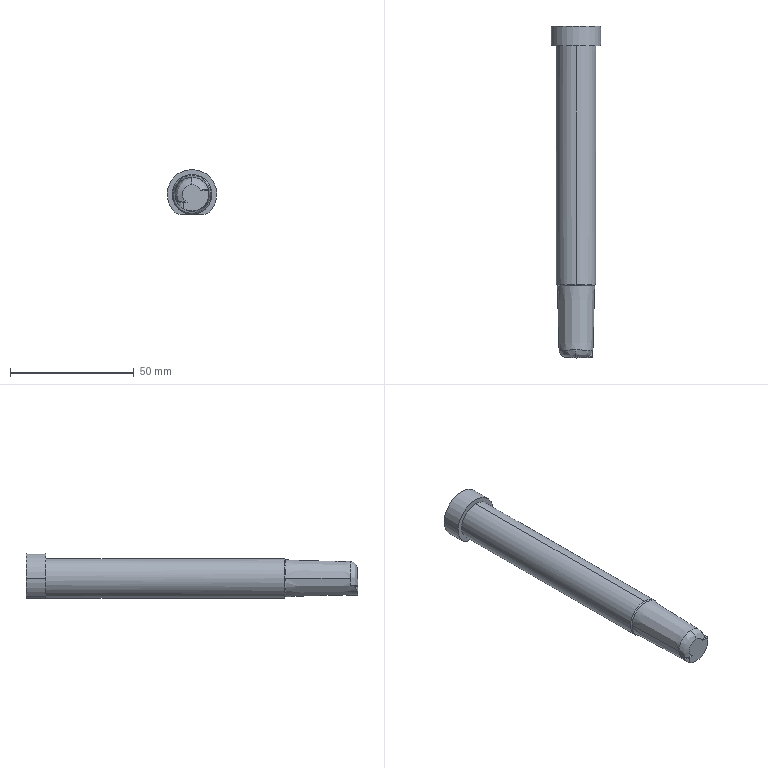Part | SolidWorks | features BaseBody 1 | 1 solid | 25 faces | box 20 x 134.117 x 18.065 mm | volume 26492 mm3 | cylinder 10 | plane 6 | spline 5 | cone 4 | commonest cylinder face diameters 20 x3 0.603 x2 6 x2 16 x2 6.033 x1
STEP:
#1=CARTESIAN_POINT('',(7.528,100.091,21.065));
#2=VERTEX_POINT('',#1);
#3=CARTESIAN_POINT('',(-7.528,100.091,21.065));
#4=VERTEX_POINT('',#3);
#5=CARTESIAN_POINT('',(0.,100.091,21.065));
#6=DIRECTION('',(0.,1.,0.));
#7=DIRECTION('',(1.,0.,0.));
#8=AXIS2_PLACEMENT_3D('',#5,#6,#7);
#9=CIRCLE('',#8,7.528);
#10=EDGE_CURVE('',#2,#4,#9,.T.);
#11=ORIENTED_EDGE('',*,*,#10,.T.);
#12=CARTESIAN_POINT('',(-8.,100.551,21.065));
#13=VERTEX_POINT('',#12);
#14=CARTESIAN_POINT('',(-8.044,100.594,21.065));
#15=DIRECTION('',(-0.7163,0.6978,0.));
#16=VECTOR('',#15,1000.);
#17=LINE('',#14,#16);
#18=EDGE_CURVE('',#4,#13,#17,.T.);
#19=ORIENTED_EDGE('',*,*,#18,.T.);
#20=CARTESIAN_POINT('',(0.,100.551,13.065));
#21=VERTEX_POINT('',#20);
#22=CARTESIAN_POINT('',(0.,100.551,21.065));
#23=DIRECTION('',(0.,1.,0.));
#24=DIRECTION('',(-1.,0.,0.));
#25=AXIS2_PLACEMENT_3D('',#22,#23,#24);
#26=CIRCLE('',#25,8.);
#27=EDGE_CURVE('',#21,#13,#26,.T.);
#28=ORIENTED_EDGE('',*,*,#27,.F.);
#29=CARTESIAN_POINT('',(8.,100.551,21.065));
#30=VERTEX_POINT('',#29);
#31=CARTESIAN_POINT('',(0.,100.551,21.065));
#32=DIRECTION('',(0.,1.,0.));
#33=DIRECTION('',(-1.,0.,0.));
#34=AXIS2_PLACEMENT_3D('',#31,#32,#33);
#35=CIRCLE('',#34,8.);
#36=EDGE_CURVE('',#30,#21,#35,.T.);
#37=ORIENTED_EDGE('',*,*,#36,.F.);
#38=CARTESIAN_POINT('',(8.044,100.594,21.065));
#39=DIRECTION('',(0.7163,0.6978,0.));
#40=VECTOR('',#39,1000.);
#41=LINE('',#38,#40);
#42=EDGE_CURVE('',#2,#30,#41,.T.);
#43=ORIENTED_EDGE('',*,*,#42,.F.);
#44=EDGE_LOOP('',(#11,#19,#28,#37,#43));
#45=FACE_OUTER_BOUND('',#44,.T.);
#46=CARTESIAN_POINT('',(0.,100.594,21.065));
#47=DIRECTION('',(0.,1.,0.));
#48=DIRECTION('',(1.,0.,0.));
#49=AXIS2_PLACEMENT_3D('',#46,#47,#48);
#50=CONICAL_SURFACE('',#49,8.044,0.7985);
#51=ADVANCED_FACE('',(#45),#50,.T.);
#52=CARTESIAN_POINT('',(-6.845,73.998,21.065));
#53=VERTEX_POINT('',#52);
#54=CARTESIAN_POINT('',(-6.191,73.956,18.149));
#55=VERTEX_POINT('',#54);
#56=CARTESIAN_POINT('',(-6.845,73.998,21.065));
#57=CARTESIAN_POINT('',(-6.845,73.991,20.559));
#58=CARTESIAN_POINT('',(-6.789,73.984,20.063));
#59=CARTESIAN_POINT('',(-6.571,73.969,19.088));
#60=CARTESIAN_POINT('',(-6.407,73.962,18.607));
#61=CARTESIAN_POINT('',(-6.191,73.956,18.149));
#62=B_SPLINE_CURVE_WITH_KNOTS('',3,(#56,#57,#58,#59,#60,#61),.UNSPECIFIED.,.F.,.F.,(4,2,4),(0.,0.001496,0.002993),.UNSPECIFIED.);
#63=EDGE_CURVE('',#53,#55,#62,.T.);
#64=ORIENTED_EDGE('',*,*,#63,.F.);
#65=CARTESIAN_POINT('',(-7.541,100.594,21.065));
#66=DIRECTION('',(-0.02618,0.9997,0.));
#67=VECTOR('',#66,1000.);
#68=LINE('',#65,#67);
#69=EDGE_CURVE('',#53,#4,#68,.T.);
#70=ORIENTED_EDGE('',*,*,#69,.T.);
#71=ORIENTED_EDGE('',*,*,#10,.F.);
#72=CARTESIAN_POINT('',(6.768,71.06,21.065));
#73=VERTEX_POINT('',#72);
#74=CARTESIAN_POINT('',(7.541,100.594,21.065));
#75=DIRECTION('',(0.02618,0.9997,0.));
#76=VECTOR('',#75,1000.);
#77=LINE('',#74,#76);
#78=EDGE_CURVE('',#73,#2,#77,.T.);
#79=ORIENTED_EDGE('',*,*,#78,.F.);
#80=CARTESIAN_POINT('',(-3.608,70.91,15.344));
#81=VERTEX_POINT('',#80);
#82=CARTESIAN_POINT('',(6.768,71.06,21.065));
#83=CARTESIAN_POINT('',(6.764,70.902,15.041));
#84=CARTESIAN_POINT('',(1.488,70.826,12.132));
#85=CARTESIAN_POINT('',(-3.608,70.91,15.344));
#86=(BOUNDED_CURVE()B_SPLINE_CURVE(3,(#82,#83,#84,#85),.UNSPECIFIED.,.F.,.F.)B_SPLINE_CURVE_WITH_KNOTS((4,4),(1.571,3.704),.UNSPECIFIED.)CURVE()GEOMETRIC_REPRESENTATION_ITEM()RATIONAL_B_SPLINE_CURVE((1.,0.6556,0.6556,1.))REPRESENTATION_ITEM(''));
#87=EDGE_CURVE('',#73,#81,#86,.T.);
#88=ORIENTED_EDGE('',*,*,#87,.T.);
#89=CARTESIAN_POINT('',(-5.995,72.237,17.859));
#90=VERTEX_POINT('',#89);
#91=CARTESIAN_POINT('',(-3.608,70.91,15.344));
#92=CARTESIAN_POINT('',(-3.879,70.914,15.515));
#93=CARTESIAN_POINT('',(-4.131,70.956,15.699));
#94=CARTESIAN_POINT('',(-4.603,71.094,16.093));
#95=CARTESIAN_POINT('',(-4.825,71.193,16.306));
#96=CARTESIAN_POINT('',(-5.224,71.428,16.737));
#97=CARTESIAN_POINT('',(-5.403,71.565,16.958));
#98=CARTESIAN_POINT('',(-5.725,71.875,17.406));
#99=CARTESIAN_POINT('',(-5.869,72.047,17.635));
#100=CARTESIAN_POINT('',(-5.995,72.237,17.859));
#101=B_SPLINE_CURVE_WITH_KNOTS('',3,(#91,#92,#93,#94,#95,#96,#97,#98,#99,#100),.UNSPECIFIED.,.F.,.F.,(4,2,2,2,4),(0.00007647,0.001021,0.001965,0.002909,0.003853),.UNSPECIFIED.);
#102=EDGE_CURVE('',#81,#90,#101,.T.);
#103=ORIENTED_EDGE('',*,*,#102,.T.);
#104=CARTESIAN_POINT('',(-6.169,73.191,18.148));
#105=VERTEX_POINT('',#104);
#106=CARTESIAN_POINT('',(-5.995,72.237,17.859));
#107=CARTESIAN_POINT('',(-6.03,72.289,17.921));
#108=CARTESIAN_POINT('',(-6.055,72.361,17.967));
#109=CARTESIAN_POINT('',(-6.097,72.513,18.04));
#110=CARTESIAN_POINT('',(-6.113,72.595,18.067));
#111=CARTESIAN_POINT('',(-6.15,72.846,18.128));
#112=CARTESIAN_POINT('',(-6.161,73.018,18.143));
#113=CARTESIAN_POINT('',(-6.169,73.191,18.148));
#114=B_SPLINE_CURVE_WITH_KNOTS('',3,(#106,#107,#108,#109,#110,#111,#112,#113),.UNSPECIFIED.,.F.,.F.,(4,2,2,4),(0.,0.0002617,0.0005235,0.001047),.UNSPECIFIED.);
#115=EDGE_CURVE('',#90,#105,#114,.T.);
#116=ORIENTED_EDGE('',*,*,#115,.T.);
#117=CARTESIAN_POINT('',(-6.173,73.305,18.149));
#118=VERTEX_POINT('',#117);
#119=CARTESIAN_POINT('',(-6.169,73.191,18.148));
#120=CARTESIAN_POINT('',(-6.17,73.229,18.149));
#121=CARTESIAN_POINT('',(-6.171,73.267,18.149));
#122=CARTESIAN_POINT('',(-6.173,73.305,18.149));
#123=B_SPLINE_CURVE_WITH_KNOTS('',3,(#119,#120,#121,#122),.UNSPECIFIED.,.F.,.F.,(4,4),(0.,0.000114),.UNSPECIFIED.);
#124=EDGE_CURVE('',#105,#118,#123,.T.);
#125=ORIENTED_EDGE('',*,*,#124,.T.);
#126=CARTESIAN_POINT('',(-6.173,73.305,18.149));
#127=CARTESIAN_POINT('',(-6.179,73.522,18.149));
#128=CARTESIAN_POINT('',(-6.185,73.739,18.149));
#129=CARTESIAN_POINT('',(-6.191,73.956,18.149));
#130=B_SPLINE_CURVE_WITH_KNOTS('',3,(#126,#127,#128,#129),.UNSPECIFIED.,.F.,.F.,(4,4),(0.03892,0.03957),.UNSPECIFIED.);
#131=EDGE_CURVE('',#118,#55,#130,.T.);
#132=ORIENTED_EDGE('',*,*,#131,.T.);
#133=EDGE_LOOP('',(#64,#70,#71,#79,#88,#103,#116,#125,#132));
#134=FACE_OUTER_BOUND('',#133,.T.);
#135=CARTESIAN_POINT('',(0.,100.594,21.065));
#136=DIRECTION('',(0.,1.,0.));
#137=DIRECTION('',(1.,0.,0.));
#138=AXIS2_PLACEMENT_3D('',#135,#136,#137);
#139=CONICAL_SURFACE('',#138,7.541,0.02618);
#140=ADVANCED_FACE('',(#134),#139,.T.);
#141=CARTESIAN_POINT('',(6.602,74.025,22.875));
#142=VERTEX_POINT('',#141);
#143=CARTESIAN_POINT('',(-0.000000001,74.099,27.913));
#144=VERTEX_POINT('',#143);
#145=CARTESIAN_POINT('',(6.602,74.025,22.875));
#146=CARTESIAN_POINT('',(6.404,74.036,23.599));
#147=CARTESIAN_POINT('',(6.095,74.045,24.272));
#148=CARTESIAN_POINT('',(5.467,74.059,25.204));
#149=CARTESIAN_POINT('',(5.233,74.063,25.495));
#150=CARTESIAN_POINT('',(4.725,74.071,26.034));
#151=CARTESIAN_POINT('',(4.45,74.075,26.282));
#152=CARTESIAN_POINT('',(3.855,74.081,26.736));
#153=CARTESIAN_POINT('',(3.54,74.084,26.938));
#154=CARTESIAN_POINT('',(2.886,74.09,27.286));
#155=CARTESIAN_POINT('',(2.546,74.092,27.433));
#156=CARTESIAN_POINT('',(1.838,74.095,27.672));
#157=CARTESIAN_POINT('',(1.473,74.097,27.763));
#158=CARTESIAN_POINT('',(0.7421,74.098,27.882));
#159=CARTESIAN_POINT('',(0.3729,74.099,27.913));
#160=CARTESIAN_POINT('',(-0.000000001,74.099,27.913));
#161=B_SPLINE_CURVE_WITH_KNOTS('',3,(#145,#146,#147,#148,#149,#150,#151,#152,#153,#154,#155,#156,#157,#158,#159,#160),.UNSPECIFIED.,.F.,.F.,(4,2,2,2,2,2,2,4),(-0.01958,-0.01736,-0.01625,-0.01514,-0.01402,-0.01291,-0.0118,-0.01069),.UNSPECIFIED.);
#162=EDGE_CURVE('',#142,#144,#161,.T.);
#163=ORIENTED_EDGE('',*,*,#162,.T.);
#164=CARTESIAN_POINT('',(-0.000000001,71.162,24.976));
#165=VERTEX_POINT('',#164);
#166=CARTESIAN_POINT('',(0.,74.178,24.897));
#167=DIRECTION('',(1.,0.,0.));
#168=DIRECTION('',(0.,0.,-1.));
#169=AXIS2_PLACEMENT_3D('',#166,#167,#168);
#170=CIRCLE('',#169,3.016);
#171=EDGE_CURVE('',#144,#165,#170,.T.);
#172=ORIENTED_EDGE('',*,*,#171,.T.);
#173=CARTESIAN_POINT('',(3.55,71.1,22.581));
#174=VERTEX_POINT('',#173);
#175=CARTESIAN_POINT('',(-0.000000001,71.162,24.976));
#176=CARTESIAN_POINT('',(1.611,71.162,24.976));
#177=CARTESIAN_POINT('',(2.947,71.139,24.075));
#178=CARTESIAN_POINT('',(3.55,71.1,22.581));
#179=(BOUNDED_CURVE()B_SPLINE_CURVE(3,(#175,#176,#177,#178),.UNSPECIFIED.,.F.,.F.)B_SPLINE_CURVE_WITH_KNOTS((4,4),(6.283,7.47),.UNSPECIFIED.)CURVE()GEOMETRIC_REPRESENTATION_ITEM()RATIONAL_B_SPLINE_CURVE((1.,0.886,0.886,1.))REPRESENTATION_ITEM(''));
#180=EDGE_CURVE('',#165,#174,#179,.T.);
#181=ORIENTED_EDGE('',*,*,#180,.T.);
#182=CARTESIAN_POINT('',(4.825,71.401,22.875));
#183=VERTEX_POINT('',#182);
#184=CARTESIAN_POINT('',(4.825,71.401,22.875));
#185=CARTESIAN_POINT('',(4.617,71.307,22.875));
#186=CARTESIAN_POINT('',(4.407,71.232,22.834));
#187=CARTESIAN_POINT('',(3.979,71.129,22.723));
#188=CARTESIAN_POINT('',(3.765,71.101,22.653));
#189=CARTESIAN_POINT('',(3.55,71.1,22.581));
#190=B_SPLINE_CURVE_WITH_KNOTS('',3,(#184,#185,#186,#187,#188,#189),.UNSPECIFIED.,.F.,.F.,(4,2,4),(0.,0.0006766,0.001353),.UNSPECIFIED.);
#191=EDGE_CURVE('',#183,#174,#190,.T.);
#192=ORIENTED_EDGE('',*,*,#191,.F.);
#193=CARTESIAN_POINT('',(4.825,71.401,22.875));
#194=CARTESIAN_POINT('',(5.078,71.515,22.875));
#195=CARTESIAN_POINT('',(5.313,71.66,22.875));
#196=CARTESIAN_POINT('',(5.746,72.019,22.875));
#197=CARTESIAN_POINT('',(5.933,72.224,22.875));
#198=CARTESIAN_POINT('',(6.169,72.568,22.875));
#199=CARTESIAN_POINT('',(6.241,72.69,22.875));
#200=CARTESIAN_POINT('',(6.364,72.94,22.875));
#201=CARTESIAN_POINT('',(6.416,73.069,22.875));
#202=CARTESIAN_POINT('',(6.545,73.464,22.875));
#203=CARTESIAN_POINT('',(6.594,73.744,22.875));
#204=CARTESIAN_POINT('',(6.602,74.025,22.875));
#205=B_SPLINE_CURVE_WITH_KNOTS('',3,(#193,#194,#195,#196,#197,#198,#199,#200,#201,#202,#203,#204),.UNSPECIFIED.,.F.,.F.,(4,2,2,2,2,4),(0.001442,0.002273,0.003104,0.003519,0.003935,0.004766),.UNSPECIFIED.);
#206=EDGE_CURVE('',#183,#142,#205,.T.);
#207=ORIENTED_EDGE('',*,*,#206,.T.);
#208=EDGE_LOOP('',(#163,#172,#181,#192,#207));
#209=FACE_OUTER_BOUND('',#208,.T.);
#210=CARTESIAN_POINT('',(6.617,74.024,22.821));
#211=CARTESIAN_POINT('',(6.524,71.107,22.873));
#212=CARTESIAN_POINT('',(3.702,71.088,22.127));
#213=CARTESIAN_POINT('',(6.425,74.035,23.544));
#214=CARTESIAN_POINT('',(6.327,71.126,23.583));
#215=CARTESIAN_POINT('',(3.595,71.098,22.531));
#216=CARTESIAN_POINT('',(6.114,74.045,24.236));
#217=CARTESIAN_POINT('',(6.014,71.143,24.26));
#218=CARTESIAN_POINT('',(3.421,71.108,22.918));
#219=CARTESIAN_POINT('',(5.285,74.063,25.482));
#220=CARTESIAN_POINT('',(5.189,71.175,25.477));
#221=CARTESIAN_POINT('',(2.957,71.127,23.616));
#222=CARTESIAN_POINT('',(4.767,74.071,26.036));
#223=CARTESIAN_POINT('',(4.677,71.189,26.017));
#224=CARTESIAN_POINT('',(2.668,71.135,23.926));
#225=CARTESIAN_POINT('',(3.581,74.085,26.949));
#226=CARTESIAN_POINT('',(3.508,71.213,26.904));
#227=CARTESIAN_POINT('',(2.004,71.148,24.437));
#228=CARTESIAN_POINT('',(2.913,74.09,27.307));
#229=CARTESIAN_POINT('',(2.852,71.222,27.251));
#230=CARTESIAN_POINT('',(1.63,71.153,24.637));
#231=CARTESIAN_POINT('',(1.496,74.097,27.789));
#232=CARTESIAN_POINT('',(1.464,71.234,27.718));
#233=CARTESIAN_POINT('',(0.8373,71.16,24.907));
#234=CARTESIAN_POINT('',(0.7483,74.099,27.913));
#235=CARTESIAN_POINT('',(0.7319,71.237,27.838));
#236=CARTESIAN_POINT('',(0.4187,71.162,24.976));
#237=CARTESIAN_POINT('',(-0.000000001,74.099,27.913));
#238=CARTESIAN_POINT('',(-0.000000001,71.237,27.838));
#239=CARTESIAN_POINT('',(-0.000000001,71.162,24.976));
#240=(BOUNDED_SURFACE()B_SPLINE_SURFACE(3,2,((#210,#211,#212),(#213,#214,#215),(#216,#217,#218),(#219,#220,#221),(#222,#223,#224),(#225,#226,#227),(#228,#229,#230),(#231,#232,#233),(#234,#235,#236),(#237,#238,#239)),.UNSPECIFIED.,.F.,.F.,.F.)B_SPLINE_SURFACE_WITH_KNOTS((4,2,2,2,4),(3,3),(4.971,5.299,5.627,5.955,6.283),(0.,1.),.UNSPECIFIED.)GEOMETRIC_REPRESENTATION_ITEM()RATIONAL_B_SPLINE_SURFACE(((1.,0.7186,1.),(1.,0.7196,1.),(1.,0.7205,1.),(1.,0.7222,1.),(1.,0.7229,1.),(1.,0.7241,1.),(1.,0.7246,1.),(1.,0.7252,1.),(1.,0.7254,1.),(1.,0.7254,1.)))REPRESENTATION_ITEM('')SURFACE());
#241=ADVANCED_FACE('',(#209),#240,.T.);
#242=CARTESIAN_POINT('',(-4.717,71.545,18.149));
#243=VERTEX_POINT('',#242);
#244=CARTESIAN_POINT('',(-5.462,72.072,18.149));
#245=VERTEX_POINT('',#244);
#246=CARTESIAN_POINT('',(-4.717,71.545,18.149));
#247=CARTESIAN_POINT('',(-4.994,71.677,18.149));
#248=CARTESIAN_POINT('',(-5.245,71.855,18.149));
#249=CARTESIAN_POINT('',(-5.462,72.072,18.149));
#250=(BOUNDED_CURVE()B_SPLINE_CURVE(3,(#246,#247,#248,#249),.UNSPECIFIED.,.F.,.F.)B_SPLINE_CURVE_WITH_KNOTS((4,4),(5.946,6.283),.UNSPECIFIED.)CURVE()GEOMETRIC_REPRESENTATION_ITEM()RATIONAL_B_SPLINE_CURVE((1.,0.9905,0.9905,1.))REPRESENTATION_ITEM(''));
#251=EDGE_CURVE('',#243,#245,#250,.T.);
#252=ORIENTED_EDGE('',*,*,#251,.T.);
#253=CARTESIAN_POINT('',(-5.675,71.859,17.859));
#254=VERTEX_POINT('',#253);
#255=CARTESIAN_POINT('',(-5.462,72.072,17.848));
#256=DIRECTION('',(0.7071,-0.7071,0.));
#257=DIRECTION('',(0.7071,0.7071,0.));
#258=AXIS2_PLACEMENT_3D('',#255,#256,#257);
#259=CIRCLE('',#258,0.3017);
#260=EDGE_CURVE('',#245,#254,#259,.T.);
#261=ORIENTED_EDGE('',*,*,#260,.T.);
#262=CARTESIAN_POINT('',(-3.543,70.976,17.856));
#263=VERTEX_POINT('',#262);
#264=CARTESIAN_POINT('',(-5.675,71.859,17.859));
#265=CARTESIAN_POINT('',(-5.102,71.286,17.859));
#266=CARTESIAN_POINT('',(-4.353,70.976,17.858));
#267=CARTESIAN_POINT('',(-3.543,70.976,17.856));
#268=(BOUNDED_CURVE()B_SPLINE_CURVE(3,(#264,#265,#266,#267),.UNSPECIFIED.,.F.,.F.)B_SPLINE_CURVE_WITH_KNOTS((4,4),(0.,0.7851),.UNSPECIFIED.)CURVE()GEOMETRIC_REPRESENTATION_ITEM()RATIONAL_B_SPLINE_CURVE((1.,0.9493,0.9493,1.))REPRESENTATION_ITEM(''));
#269=EDGE_CURVE('',#254,#263,#268,.T.);
#270=ORIENTED_EDGE('',*,*,#269,.T.);
#271=CARTESIAN_POINT('',(-3.543,71.103,18.094));
#272=VERTEX_POINT('',#271);
#273=CARTESIAN_POINT('',(-3.543,71.277,17.848));
#274=DIRECTION('',(1.,0.,0.));
#275=DIRECTION('',(0.,0.,1.));
#276=AXIS2_PLACEMENT_3D('',#273,#274,#275);
#277=CIRCLE('',#276,0.3017);
#278=EDGE_CURVE('',#272,#263,#277,.T.);
#279=ORIENTED_EDGE('',*,*,#278,.F.);
#280=CARTESIAN_POINT('',(-3.543,71.103,18.094));
#281=CARTESIAN_POINT('',(-3.749,71.144,18.123));
#282=CARTESIAN_POINT('',(-3.951,71.199,18.134));
#283=CARTESIAN_POINT('',(-4.343,71.345,18.148));
#284=CARTESIAN_POINT('',(-4.535,71.436,18.149));
#285=CARTESIAN_POINT('',(-4.717,71.545,18.149));
#286=B_SPLINE_CURVE_WITH_KNOTS('',3,(#280,#281,#282,#283,#284,#285),.UNSPECIFIED.,.F.,.F.,(4,2,4),(0.0004358,0.001068,0.0017),.UNSPECIFIED.);
#287=EDGE_CURVE('',#272,#243,#286,.T.);
#288=ORIENTED_EDGE('',*,*,#287,.T.);
#289=EDGE_LOOP('',(#252,#261,#270,#279,#288));
#290=FACE_OUTER_BOUND('',#289,.T.);
#291=CARTESIAN_POINT('',(-3.543,71.277,18.149));
#292=CARTESIAN_POINT('',(-3.543,70.983,18.149));
#293=CARTESIAN_POINT('',(-3.543,70.976,17.856));
#294=CARTESIAN_POINT('',(-3.898,71.277,18.149));
#295=CARTESIAN_POINT('',(-3.936,70.984,18.149));
#296=CARTESIAN_POINT('',(-3.937,70.976,17.857));
#297=CARTESIAN_POINT('',(-4.253,71.348,18.149));
#298=CARTESIAN_POINT('',(-4.329,71.063,18.149));
#299=CARTESIAN_POINT('',(-4.332,71.054,17.857));
#300=CARTESIAN_POINT('',(-4.909,71.62,18.149));
#301=CARTESIAN_POINT('',(-5.056,71.365,18.149));
#302=CARTESIAN_POINT('',(-5.061,71.356,17.858));
#303=CARTESIAN_POINT('',(-5.21,71.821,18.149));
#304=CARTESIAN_POINT('',(-5.389,71.588,18.149));
#305=CARTESIAN_POINT('',(-5.396,71.58,17.859));
#306=CARTESIAN_POINT('',(-5.462,72.072,18.149));
#307=CARTESIAN_POINT('',(-5.667,71.867,18.149));
#308=CARTESIAN_POINT('',(-5.675,71.859,17.859));
#309=(BOUNDED_SURFACE()B_SPLINE_SURFACE(3,2,((#291,#292,#293),(#294,#295,#296),(#297,#298,#299),(#300,#301,#302),(#303,#304,#305),(#306,#307,#308)),.UNSPECIFIED.,.F.,.F.,.F.)B_SPLINE_SURFACE_WITH_KNOTS((4,2,4),(3,3),(5.498,5.891,6.283),(0.,1.),.UNSPECIFIED.)GEOMETRIC_REPRESENTATION_ITEM()RATIONAL_B_SPLINE_SURFACE(((1.,0.7163,1.),(1.,0.7175,1.),(1.,0.7185,1.),(1.,0.7197,1.),(1.,0.7201,1.),(1.,0.7201,1.)))REPRESENTATION_ITEM('')SURFACE());
#310=ADVANCED_FACE('',(#290),#309,.T.);
#311=CARTESIAN_POINT('',(0.,100.551,29.065));
#312=VERTEX_POINT('',#311);
#313=CARTESIAN_POINT('',(0.,100.551,21.065));
#314=DIRECTION('',(0.,1.,0.));
#315=DIRECTION('',(-1.,0.,0.));
#316=AXIS2_PLACEMENT_3D('',#313,#314,#315);
#317=CIRCLE('',#316,8.);
#318=EDGE_CURVE('',#312,#30,#317,.T.);
#319=ORIENTED_EDGE('',*,*,#318,.T.);
#320=ORIENTED_EDGE('',*,*,#36,.T.);
#321=CARTESIAN_POINT('',(0.,197.,13.065));
#322=VERTEX_POINT('',#321);
#323=CARTESIAN_POINT('',(0.,100.594,13.065));
#324=DIRECTION('',(0.,1.,0.));
#325=VECTOR('',#324,1000.);
#326=LINE('',#323,#325);
#327=EDGE_CURVE('',#21,#322,#326,.T.);
#328=ORIENTED_EDGE('',*,*,#327,.T.);
#329=CARTESIAN_POINT('',(0.,197.,29.065));
#330=VERTEX_POINT('',#329);
#331=CARTESIAN_POINT('',(0.,197.,21.065));
#332=DIRECTION('',(0.,1.,0.));
#333=DIRECTION('',(1.,0.,0.));
#334=AXIS2_PLACEMENT_3D('',#331,#332,#333);
#335=CIRCLE('',#334,8.);
#336=EDGE_CURVE('',#330,#322,#335,.T.);
#337=ORIENTED_EDGE('',*,*,#336,.F.);
#338=CARTESIAN_POINT('',(0.,100.594,29.065));
#339=DIRECTION('',(0.,1.,0.));
#340=VECTOR('',#339,1000.);
#341=LINE('',#338,#340);
#342=EDGE_CURVE('',#312,#330,#341,.T.);
#343=ORIENTED_EDGE('',*,*,#342,.F.);
#344=EDGE_LOOP('',(#319,#320,#328,#337,#343));
#345=FACE_OUTER_BOUND('',#344,.T.);
#346=CARTESIAN_POINT('',(0.,100.594,21.065));
#347=DIRECTION('',(0.,1.,0.));
#348=DIRECTION('',(0.,0.,1.));
#349=AXIS2_PLACEMENT_3D('',#346,#347,#348);
#350=CYLINDRICAL_SURFACE('',#349,8.);
#351=ADVANCED_FACE('',(#345),#350,.T.);
#352=CARTESIAN_POINT('',(10.,205.,21.065));
#353=VERTEX_POINT('',#352);
#354=CARTESIAN_POINT('',(-10.,205.,21.065));
#355=VERTEX_POINT('',#354);
#356=CARTESIAN_POINT('',(0.,205.,21.065));
#357=DIRECTION('',(0.,-1.,0.));
#358=DIRECTION('',(1.,0.,0.));
#359=AXIS2_PLACEMENT_3D('',#356,#357,#358);
#360=CIRCLE('',#359,10.);
#361=EDGE_CURVE('',#353,#355,#360,.T.);
#362=ORIENTED_EDGE('',*,*,#361,.T.);
#363=CARTESIAN_POINT('',(-10.,197.,21.065));
#364=VERTEX_POINT('',#363);
#365=CARTESIAN_POINT('',(-10.,205.,21.065));
#366=DIRECTION('',(0.,-1.,0.));
#367=VECTOR('',#366,1000.);
#368=LINE('',#365,#367);
#369=EDGE_CURVE('',#355,#364,#368,.T.);
#370=ORIENTED_EDGE('',*,*,#369,.T.);
#371=CARTESIAN_POINT('',(10.,197.,21.065));
#372=VERTEX_POINT('',#371);
#373=CARTESIAN_POINT('',(0.,197.,21.065));
#374=DIRECTION('',(0.,-1.,0.));
#375=DIRECTION('',(1.,0.,0.));
#376=AXIS2_PLACEMENT_3D('',#373,#374,#375);
#377=CIRCLE('',#376,10.);
#378=EDGE_CURVE('',#372,#364,#377,.T.);
#379=ORIENTED_EDGE('',*,*,#378,.F.);
#380=CARTESIAN_POINT('',(10.,205.,21.065));
#381=DIRECTION('',(0.,-1.,0.));
#382=VECTOR('',#381,1000.);
#383=LINE('',#380,#382);
#384=EDGE_CURVE('',#353,#372,#383,.T.);
#385=ORIENTED_EDGE('',*,*,#384,.F.);
#386=EDGE_LOOP('',(#362,#370,#379,#385));
#387=FACE_OUTER_BOUND('',#386,.T.);
#388=CARTESIAN_POINT('',(0.,205.,21.065));
#389=DIRECTION('',(0.,-1.,0.));
#390=DIRECTION('',(1.,0.,0.));
#391=AXIS2_PLACEMENT_3D('',#388,#389,#390);
#392=CYLINDRICAL_SURFACE('',#391,10.);
#393=ADVANCED_FACE('',(#387),#392,.T.);
#394=CARTESIAN_POINT('',(6.902,205.,13.829));
#395=VERTEX_POINT('',#394);
#396=CARTESIAN_POINT('',(0.,205.,21.065));
#397=DIRECTION('',(0.,-1.,0.));
#398=DIRECTION('',(1.,0.,0.));
#399=AXIS2_PLACEMENT_3D('',#396,#397,#398);
#400=CIRCLE('',#399,10.);
#401=EDGE_CURVE('',#395,#353,#400,.T.);
#402=ORIENTED_EDGE('',*,*,#401,.T.);
#403=ORIENTED_EDGE('',*,*,#384,.T.);
#404=CARTESIAN_POINT('',(6.902,197.,13.829));
#405=VERTEX_POINT('',#404);
#406=CARTESIAN_POINT('',(0.,197.,21.065));
#407=DIRECTION('',(0.,-1.,0.));
#408=DIRECTION('',(1.,0.,0.));
#409=AXIS2_PLACEMENT_3D('',#406,#407,#408);
#410=CIRCLE('',#409,10.);
#411=EDGE_CURVE('',#405,#372,#410,.T.);
#412=ORIENTED_EDGE('',*,*,#411,.F.);
#413=CARTESIAN_POINT('',(6.902,205.,13.829));
#414=DIRECTION('',(0.,1.,0.));
#415=VECTOR('',#414,1000.);
#416=LINE('',#413,#415);
#417=EDGE_CURVE('',#405,#395,#416,.T.);
#418=ORIENTED_EDGE('',*,*,#417,.T.);
#419=EDGE_LOOP('',(#402,#403,#412,#418));
#420=FACE_OUTER_BOUND('',#419,.T.);
#421=CARTESIAN_POINT('',(0.,205.,21.065));
#422=DIRECTION('',(0.,-1.,0.));
#423=DIRECTION('',(1.,0.,0.));
#424=AXIS2_PLACEMENT_3D('',#421,#422,#423);
#425=CYLINDRICAL_SURFACE('',#424,10.);
#426=ADVANCED_FACE('',(#420),#425,.T.);
#427=ORIENTED_EDGE('',*,*,#336,.T.);
#428=CARTESIAN_POINT('',(0.,197.,21.065));
#429=DIRECTION('',(0.,1.,0.));
#430=DIRECTION('',(1.,0.,0.));
#431=AXIS2_PLACEMENT_3D('',#428,#429,#430);
#432=CIRCLE('',#431,8.);
#433=EDGE_CURVE('',#322,#330,#432,.T.);
#434=ORIENTED_EDGE('',*,*,#433,.T.);
#435=EDGE_LOOP('',(#427,#434));
#436=FACE_BOUND('',#435,.T.);
#437=ORIENTED_EDGE('',*,*,#411,.T.);
#438=ORIENTED_EDGE('',*,*,#378,.T.);
#439=CARTESIAN_POINT('',(-6.902,197.,13.829));
#440=VERTEX_POINT('',#439);
#441=CARTESIAN_POINT('',(0.,197.,21.065));
#442=DIRECTION('',(0.,-1.,0.));
#443=DIRECTION('',(1.,0.,0.));
#444=AXIS2_PLACEMENT_3D('',#441,#442,#443);
#445=CIRCLE('',#444,10.);
#446=EDGE_CURVE('',#364,#440,#445,.T.);
#447=ORIENTED_EDGE('',*,*,#446,.T.);
#448=CARTESIAN_POINT('',(-4.832,197.,13.));
#449=VERTEX_POINT('',#448);
#450=CARTESIAN_POINT('',(-4.832,197.,16.));
#451=DIRECTION('',(0.,-1.,0.));
#452=DIRECTION('',(1.,0.,0.));
#453=AXIS2_PLACEMENT_3D('',#450,#451,#452);
#454=CIRCLE('',#453,3.);
#455=EDGE_CURVE('',#440,#449,#454,.T.);
#456=ORIENTED_EDGE('',*,*,#455,.T.);
#457=CARTESIAN_POINT('',(4.832,197.,13.));
#458=VERTEX_POINT('',#457);
#459=CARTESIAN_POINT('',(0.,197.,13.));
#460=DIRECTION('',(1.,0.,0.));
#461=VECTOR('',#460,1000.);
#462=LINE('',#459,#461);
#463=EDGE_CURVE('',#449,#458,#462,.T.);
#464=ORIENTED_EDGE('',*,*,#463,.T.);
#465=CARTESIAN_POINT('',(4.832,197.,16.));
#466=DIRECTION('',(0.,-1.,0.));
#467=DIRECTION('',(1.,0.,0.));
#468=AXIS2_PLACEMENT_3D('',#465,#466,#467);
#469=CIRCLE('',#468,3.);
#470=EDGE_CURVE('',#458,#405,#469,.T.);
#471=ORIENTED_EDGE('',*,*,#470,.T.);
#472=EDGE_LOOP('',(#437,#438,#447,#456,#464,#471));
#473=FACE_OUTER_BOUND('',#472,.T.);
#474=CARTESIAN_POINT('',(0.,197.,21.065));
#475=DIRECTION('',(0.,-1.,0.));
#476=DIRECTION('',(1.,0.,0.));
#477=AXIS2_PLACEMENT_3D('',#474,#475,#476);
#478=PLANE('',#477);
#479=ADVANCED_FACE('',(#436,#473),#478,.T.);
#480=ORIENTED_EDGE('',*,*,#369,.F.);
#481=CARTESIAN_POINT('',(-6.902,205.,13.829));
#482=VERTEX_POINT('',#481);
#483=CARTESIAN_POINT('',(0.,205.,21.065));
#484=DIRECTION('',(0.,-1.,0.));
#485=DIRECTION('',(1.,0.,0.));
#486=AXIS2_PLACEMENT_3D('',#483,#484,#485);
#487=CIRCLE('',#486,10.);
#488=EDGE_CURVE('',#355,#482,#487,.T.);
#489=ORIENTED_EDGE('',*,*,#488,.T.);
#490=CARTESIAN_POINT('',(-6.902,205.,13.829));
#491=DIRECTION('',(0.,-1.,0.));
#492=VECTOR('',#491,1000.);
#493=LINE('',#490,#492);
#494=EDGE_CURVE('',#482,#440,#493,.T.);
#495=ORIENTED_EDGE('',*,*,#494,.T.);
#496=ORIENTED_EDGE('',*,*,#446,.F.);
#497=EDGE_LOOP('',(#480,#489,#495,#496));
#498=FACE_OUTER_BOUND('',#497,.T.);
#499=CARTESIAN_POINT('',(0.,205.,21.065));
#500=DIRECTION('',(0.,-1.,0.));
#501=DIRECTION('',(1.,0.,0.));
#502=AXIS2_PLACEMENT_3D('',#499,#500,#501);
#503=CYLINDRICAL_SURFACE('',#502,10.);
#504=ADVANCED_FACE('',(#498),#503,.T.);
#505=CARTESIAN_POINT('',(4.832,205.,13.));
#506=VERTEX_POINT('',#505);
#507=CARTESIAN_POINT('',(-4.832,205.,13.));
#508=VERTEX_POINT('',#507);
#509=CARTESIAN_POINT('',(265.,205.,13.));
#510=DIRECTION('',(-1.,0.,0.));
#511=VECTOR('',#510,1000.);
#512=LINE('',#509,#511);
#513=EDGE_CURVE('',#506,#508,#512,.T.);
#514=ORIENTED_EDGE('',*,*,#513,.T.);
#515=CARTESIAN_POINT('',(-4.832,205.,16.));
#516=DIRECTION('',(0.,1.,0.));
#517=DIRECTION('',(-1.,0.,0.));
#518=AXIS2_PLACEMENT_3D('',#515,#516,#517);
#519=CIRCLE('',#518,3.);
#520=EDGE_CURVE('',#508,#482,#519,.T.);
#521=ORIENTED_EDGE('',*,*,#520,.T.);
#522=ORIENTED_EDGE('',*,*,#488,.F.);
#523=ORIENTED_EDGE('',*,*,#361,.F.);
#524=ORIENTED_EDGE('',*,*,#401,.F.);
#525=CARTESIAN_POINT('',(4.832,205.,16.));
#526=DIRECTION('',(0.,1.,0.));
#527=DIRECTION('',(-1.,0.,0.));
#528=AXIS2_PLACEMENT_3D('',#525,#526,#527);
#529=CIRCLE('',#528,3.);
#530=EDGE_CURVE('',#395,#506,#529,.T.);
#531=ORIENTED_EDGE('',*,*,#530,.T.);
#532=EDGE_LOOP('',(#514,#521,#522,#523,#524,#531));
#533=FACE_OUTER_BOUND('',#532,.T.);
#534=CARTESIAN_POINT('',(265.,205.,-70.));
#535=DIRECTION('',(0.,1.,0.));
#536=DIRECTION('',(-1.,0.,0.));
#537=AXIS2_PLACEMENT_3D('',#534,#535,#536);
#538=PLANE('',#537);
#539=ADVANCED_FACE('',(#533),#538,.T.);
#540=ORIENTED_EDGE('',*,*,#327,.F.);
#541=ORIENTED_EDGE('',*,*,#27,.T.);
#542=CARTESIAN_POINT('',(0.,100.551,21.065));
#543=DIRECTION('',(0.,1.,0.));
#544=DIRECTION('',(-1.,0.,0.));
#545=AXIS2_PLACEMENT_3D('',#542,#543,#544);
#546=CIRCLE('',#545,8.);
#547=EDGE_CURVE('',#13,#312,#546,.T.);
#548=ORIENTED_EDGE('',*,*,#547,.T.);
#549=ORIENTED_EDGE('',*,*,#342,.T.);
#550=ORIENTED_EDGE('',*,*,#433,.F.);
#551=EDGE_LOOP('',(#540,#541,#548,#549,#550));
#552=FACE_OUTER_BOUND('',#551,.T.);
#553=CARTESIAN_POINT('',(0.,100.594,21.065));
#554=DIRECTION('',(0.,1.,0.));
#555=DIRECTION('',(0.,0.,1.));
#556=AXIS2_PLACEMENT_3D('',#553,#554,#555);
#557=CYLINDRICAL_SURFACE('',#556,8.);
#558=ADVANCED_FACE('',(#552),#557,.T.);
#559=CARTESIAN_POINT('',(-1.957,70.976,17.856));
#560=VERTEX_POINT('',#559);
#561=CARTESIAN_POINT('',(-1.957,70.976,17.856));
#562=CARTESIAN_POINT('',(-2.223,70.977,17.889));
#563=CARTESIAN_POINT('',(-2.49,70.983,17.929));
#564=CARTESIAN_POINT('',(-3.018,71.021,18.013));
#565=CARTESIAN_POINT('',(-3.281,71.051,18.057));
#566=CARTESIAN_POINT('',(-3.543,71.103,18.094));
#567=B_SPLINE_CURVE_WITH_KNOTS('',3,(#561,#562,#563,#564,#565,#566),.UNSPECIFIED.,.F.,.F.,(4,2,4),(-0.001608,-0.0008041,0.),.UNSPECIFIED.);
#568=EDGE_CURVE('',#560,#272,#567,.T.);
#569=ORIENTED_EDGE('',*,*,#568,.T.);
#570=ORIENTED_EDGE('',*,*,#278,.T.);
#571=CARTESIAN_POINT('',(18.02,70.976,17.856));
#572=DIRECTION('',(1.,0.,0.));
#573=VECTOR('',#572,1000.);
#574=LINE('',#571,#573);
#575=EDGE_CURVE('',#263,#560,#574,.T.);
#576=ORIENTED_EDGE('',*,*,#575,.T.);
#577=EDGE_LOOP('',(#569,#570,#576));
#578=FACE_OUTER_BOUND('',#577,.T.);
#579=CARTESIAN_POINT('',(18.02,71.277,17.848));
#580=DIRECTION('',(1.,0.,0.));
#581=DIRECTION('',(0.,0.,1.));
#582=AXIS2_PLACEMENT_3D('',#579,#580,#581);
#583=CYLINDRICAL_SURFACE('',#582,0.3017);
#584=ADVANCED_FACE('',(#578),#583,.T.);
#585=ORIENTED_EDGE('',*,*,#124,.F.);
#586=CARTESIAN_POINT('',(-6.139,73.2,18.149));
#587=VERTEX_POINT('',#586);
#588=CARTESIAN_POINT('',(-6.139,73.2,17.848));
#589=DIRECTION('',(0.2913,-0.9566,0.));
#590=DIRECTION('',(-0.9566,-0.2913,0.));
#591=AXIS2_PLACEMENT_3D('',#588,#589,#590);
#592=CIRCLE('',#591,0.3016);
#593=EDGE_CURVE('',#587,#105,#592,.T.);
#594=ORIENTED_EDGE('',*,*,#593,.F.);
#595=CARTESIAN_POINT('',(-6.139,73.2,18.149));
#596=CARTESIAN_POINT('',(-6.149,73.235,18.149));
#597=CARTESIAN_POINT('',(-6.161,73.27,18.149));
#598=CARTESIAN_POINT('',(-6.173,73.305,18.149));
#599=(BOUNDED_CURVE()B_SPLINE_CURVE(3,(#595,#596,#597,#598),.UNSPECIFIED.,.F.,.F.)B_SPLINE_CURVE_WITH_KNOTS((4,4),(2.652,2.685),.UNSPECIFIED.)CURVE()GEOMETRIC_REPRESENTATION_ITEM()RATIONAL_B_SPLINE_CURVE((1.,0.9999,0.9999,1.))REPRESENTATION_ITEM(''));
#600=EDGE_CURVE('',#587,#118,#599,.T.);
#601=ORIENTED_EDGE('',*,*,#600,.T.);
#602=EDGE_LOOP('',(#585,#594,#601));
#603=FACE_OUTER_BOUND('',#602,.T.);
#604=CARTESIAN_POINT('',(-6.202,73.296,18.148));
#605=CARTESIAN_POINT('',(-6.188,73.301,18.149));
#606=CARTESIAN_POINT('',(-6.173,73.306,18.149));
#607=CARTESIAN_POINT('',(-6.191,73.261,18.148));
#608=CARTESIAN_POINT('',(-6.176,73.266,18.149));
#609=CARTESIAN_POINT('',(-6.161,73.271,18.149));
#610=CARTESIAN_POINT('',(-6.179,73.226,18.148));
#611=CARTESIAN_POINT('',(-6.164,73.231,18.149));
#612=CARTESIAN_POINT('',(-6.149,73.236,18.149));
#613=CARTESIAN_POINT('',(-6.169,73.191,18.148));
#614=CARTESIAN_POINT('',(-6.154,73.196,18.149));
#615=CARTESIAN_POINT('',(-6.139,73.2,18.149));
#616=(BOUNDED_SURFACE()B_SPLINE_SURFACE(3,2,((#604,#605,#606),(#607,#608,#609),(#610,#611,#612),(#613,#614,#615)),.UNSPECIFIED.,.F.,.F.,.F.)B_SPLINE_SURFACE_WITH_KNOTS((4,4),(3,3),(3.598,3.631),(0.9267,1.),.UNSPECIFIED.)GEOMETRIC_REPRESENTATION_ITEM()RATIONAL_B_SPLINE_SURFACE(((0.9618,0.9794,1.),(0.9618,0.9794,1.),(0.9618,0.9794,1.),(0.9618,0.9794,1.)))REPRESENTATION_ITEM('')SURFACE());
#617=ADVANCED_FACE('',(#603),#616,.T.);
#618=ORIENTED_EDGE('',*,*,#260,.F.);
#619=CARTESIAN_POINT('',(-5.462,72.072,18.149));
#620=CARTESIAN_POINT('',(-5.778,72.389,18.149));
#621=CARTESIAN_POINT('',(-6.008,72.772,18.149));
#622=CARTESIAN_POINT('',(-6.139,73.2,18.149));
#623=(BOUNDED_CURVE()B_SPLINE_CURVE(3,(#619,#620,#621,#622),.UNSPECIFIED.,.F.,.F.)B_SPLINE_CURVE_WITH_KNOTS((4,4),(0.,0.4895),.UNSPECIFIED.)CURVE()GEOMETRIC_REPRESENTATION_ITEM()RATIONAL_B_SPLINE_CURVE((1.,0.9801,0.9801,1.))REPRESENTATION_ITEM(''));
#624=EDGE_CURVE('',#245,#587,#623,.T.);
#625=ORIENTED_EDGE('',*,*,#624,.T.);
#626=ORIENTED_EDGE('',*,*,#593,.T.);
#627=ORIENTED_EDGE('',*,*,#115,.F.);
#628=CARTESIAN_POINT('',(-5.995,72.237,17.859));
#629=CARTESIAN_POINT('',(-5.899,72.102,17.859));
#630=CARTESIAN_POINT('',(-5.792,71.976,17.859));
#631=CARTESIAN_POINT('',(-5.675,71.859,17.859));
#632=(BOUNDED_CURVE()B_SPLINE_CURVE(3,(#628,#629,#630,#631),.UNSPECIFIED.,.F.,.F.)B_SPLINE_CURVE_WITH_KNOTS((4,4),(6.119,6.283),.UNSPECIFIED.)CURVE()GEOMETRIC_REPRESENTATION_ITEM()RATIONAL_B_SPLINE_CURVE((1.,0.9978,0.9978,1.))REPRESENTATION_ITEM(''));
#633=EDGE_CURVE('',#90,#254,#632,.T.);
#634=ORIENTED_EDGE('',*,*,#633,.T.);
#635=EDGE_LOOP('',(#618,#625,#626,#627,#634));
#636=FACE_OUTER_BOUND('',#635,.T.);
#637=CARTESIAN_POINT('',(-5.462,72.072,18.149));
#638=CARTESIAN_POINT('',(-5.667,71.867,18.149));
#639=CARTESIAN_POINT('',(-5.675,71.859,17.859));
#640=CARTESIAN_POINT('',(-5.775,72.386,18.149));
#641=CARTESIAN_POINT('',(-6.014,72.214,18.149));
#642=CARTESIAN_POINT('',(-6.023,72.207,17.859));
#643=CARTESIAN_POINT('',(-6.009,72.776,18.149));
#644=CARTESIAN_POINT('',(-6.274,72.646,18.149));
#645=CARTESIAN_POINT('',(-6.284,72.641,17.858));
#646=CARTESIAN_POINT('',(-6.139,73.2,18.149));
#647=CARTESIAN_POINT('',(-6.418,73.115,18.149));
#648=CARTESIAN_POINT('',(-6.427,73.113,17.857));
#649=(BOUNDED_SURFACE()B_SPLINE_SURFACE(3,2,((#637,#638,#639),(#640,#641,#642),(#643,#644,#645),(#646,#647,#648)),.UNSPECIFIED.,.F.,.F.,.F.)B_SPLINE_SURFACE_WITH_KNOTS((4,4),(3,3),(0.,0.4895),(0.,1.),.UNSPECIFIED.)GEOMETRIC_REPRESENTATION_ITEM()RATIONAL_B_SPLINE_SURFACE(((1.,0.7201,1.),(1.,0.7201,1.),(1.,0.7196,1.),(1.,0.7186,1.)))REPRESENTATION_ITEM('')SURFACE());
#650=ADVANCED_FACE('',(#636),#649,.T.);
#651=ORIENTED_EDGE('',*,*,#102,.F.);
#652=CARTESIAN_POINT('',(-3.773,70.746,9.067));
#653=DIRECTION('',(0.02617,0.02617,0.9993));
#654=VECTOR('',#653,1000.);
#655=LINE('',#652,#654);
#656=EDGE_CURVE('',#81,#263,#655,.T.);
#657=ORIENTED_EDGE('',*,*,#656,.T.);
#658=ORIENTED_EDGE('',*,*,#269,.F.);
#659=ORIENTED_EDGE('',*,*,#633,.F.);
#660=EDGE_LOOP('',(#651,#657,#658,#659));
#661=FACE_OUTER_BOUND('',#660,.T.);
#662=CARTESIAN_POINT('',(-3.532,74.002,18.198));
#663=DIRECTION('',(-0.02617,-0.02617,-0.9993));
#664=DIRECTION('',(0.9997,0.,-0.02618));
#665=AXIS2_PLACEMENT_3D('',#662,#663,#664);
#666=CYLINDRICAL_SURFACE('',#665,3.016);
#667=ADVANCED_FACE('',(#661),#666,.T.);
#668=CARTESIAN_POINT('',(6.597,71.1,22.581));
#669=VERTEX_POINT('',#668);
#670=CARTESIAN_POINT('',(6.597,71.1,22.581));
#671=CARTESIAN_POINT('',(6.711,71.086,22.084));
#672=CARTESIAN_POINT('',(6.768,71.073,21.576));
#673=CARTESIAN_POINT('',(6.768,71.06,21.065));
#674=(BOUNDED_CURVE()B_SPLINE_CURVE(3,(#670,#671,#672,#673),.UNSPECIFIED.,.F.,.F.)B_SPLINE_CURVE_WITH_KNOTS((4,4),(1.346,1.571),.UNSPECIFIED.)CURVE()GEOMETRIC_REPRESENTATION_ITEM()RATIONAL_B_SPLINE_CURVE((1.,0.9958,0.9958,1.))REPRESENTATION_ITEM(''));
#675=EDGE_CURVE('',#669,#73,#674,.T.);
#676=ORIENTED_EDGE('',*,*,#675,.F.);
#677=CARTESIAN_POINT('',(18.02,71.1,22.581));
#678=DIRECTION('',(1.,0.,0.));
#679=VECTOR('',#678,1000.);
#680=LINE('',#677,#679);
#681=EDGE_CURVE('',#174,#669,#680,.T.);
#682=ORIENTED_EDGE('',*,*,#681,.F.);
#683=ORIENTED_EDGE('',*,*,#180,.F.);
#684=CARTESIAN_POINT('',(-1.957,70.976,17.856));
#685=CARTESIAN_POINT('',(-6.106,71.04,20.322));
#686=CARTESIAN_POINT('',(-4.826,71.162,24.976));
#687=CARTESIAN_POINT('',(-0.000000001,71.162,24.976));
#688=(BOUNDED_CURVE()B_SPLINE_CURVE(3,(#684,#685,#686,#687),.UNSPECIFIED.,.F.,.F.)B_SPLINE_CURVE_WITH_KNOTS((4,4),(3.678,6.283),.UNSPECIFIED.)CURVE()GEOMETRIC_REPRESENTATION_ITEM()RATIONAL_B_SPLINE_CURVE((1.,0.51,0.51,1.))REPRESENTATION_ITEM(''));
#689=EDGE_CURVE('',#560,#165,#688,.T.);
#690=ORIENTED_EDGE('',*,*,#689,.F.);
#691=ORIENTED_EDGE('',*,*,#575,.F.);
#692=ORIENTED_EDGE('',*,*,#656,.F.);
#693=ORIENTED_EDGE('',*,*,#87,.F.);
#694=EDGE_LOOP('',(#676,#682,#683,#690,#691,#692,#693));
#695=FACE_OUTER_BOUND('',#694,.T.);
#696=CARTESIAN_POINT('',(18.02,70.731,8.496));
#697=DIRECTION('',(0.,-0.9997,0.02618));
#698=DIRECTION('',(0.,-0.02618,-0.9997));
#699=AXIS2_PLACEMENT_3D('',#696,#697,#698);
#700=PLANE('',#699);
#701=ADVANCED_FACE('',(#695),#700,.T.);
#702=CARTESIAN_POINT('',(6.531,71.401,22.875));
#703=VERTEX_POINT('',#702);
#704=CARTESIAN_POINT('',(6.531,71.401,22.875));
#705=CARTESIAN_POINT('',(6.528,71.322,22.875));
#706=CARTESIAN_POINT('',(6.536,71.244,22.842));
#707=CARTESIAN_POINT('',(6.561,71.134,22.734));
#708=CARTESIAN_POINT('',(6.579,71.102,22.658));
#709=CARTESIAN_POINT('',(6.597,71.1,22.581));
#710=B_SPLINE_CURVE_WITH_KNOTS('',3,(#704,#705,#706,#707,#708,#709),.UNSPECIFIED.,.F.,.F.,(4,2,4),(0.00009623,0.0003312,0.0005662),.UNSPECIFIED.);
#711=EDGE_CURVE('',#703,#669,#710,.T.);
#712=ORIENTED_EDGE('',*,*,#711,.F.);
#713=CARTESIAN_POINT('',(-178.728,71.401,22.875));
#714=DIRECTION('',(-1.,0.,0.));
#715=VECTOR('',#714,1000.);
#716=LINE('',#713,#715);
#717=EDGE_CURVE('',#703,#183,#716,.T.);
#718=ORIENTED_EDGE('',*,*,#717,.T.);
#719=ORIENTED_EDGE('',*,*,#191,.T.);
#720=ORIENTED_EDGE('',*,*,#681,.T.);
#721=EDGE_LOOP('',(#712,#718,#719,#720));
#722=FACE_OUTER_BOUND('',#721,.T.);
#723=CARTESIAN_POINT('',(-178.728,71.401,22.573));
#724=DIRECTION('',(-1.,0.,0.));
#725=DIRECTION('',(0.,0.,-1.));
#726=AXIS2_PLACEMENT_3D('',#723,#724,#725);
#727=CYLINDRICAL_SURFACE('',#726,0.3017);
#728=ADVANCED_FACE('',(#722),#727,.T.);
#729=ORIENTED_EDGE('',*,*,#717,.F.);
#730=CARTESIAN_POINT('',(6.531,71.401,22.875));
#731=CARTESIAN_POINT('',(6.554,72.276,22.875));
#732=CARTESIAN_POINT('',(6.578,73.15,22.875));
#733=CARTESIAN_POINT('',(6.602,74.025,22.875));
#734=B_SPLINE_CURVE_WITH_KNOTS('',3,(#730,#731,#732,#733),.UNSPECIFIED.,.F.,.F.,(4,4),(0.06626,0.06888),.UNSPECIFIED.);
#735=EDGE_CURVE('',#703,#142,#734,.T.);
#736=ORIENTED_EDGE('',*,*,#735,.T.);
#737=ORIENTED_EDGE('',*,*,#206,.F.);
#738=EDGE_LOOP('',(#729,#736,#737));
#739=FACE_OUTER_BOUND('',#738,.T.);
#740=CARTESIAN_POINT('',(-178.728,104.314,22.875));
#741=DIRECTION('',(0.,0.,-1.));
#742=DIRECTION('',(1.,0.,0.));
#743=AXIS2_PLACEMENT_3D('',#740,#741,#742);
#744=PLANE('',#743);
#745=ADVANCED_FACE('',(#739),#744,.F.);
#746=ORIENTED_EDGE('',*,*,#171,.F.);
#747=CARTESIAN_POINT('',(-0.000000001,74.099,27.913));
#748=CARTESIAN_POINT('',(-0.2245,74.099,27.913));
#749=CARTESIAN_POINT('',(-0.4511,74.099,27.901));
#750=CARTESIAN_POINT('',(-0.8975,74.098,27.857));
#751=CARTESIAN_POINT('',(-1.118,74.097,27.824));
#752=CARTESIAN_POINT('',(-1.774,74.096,27.694));
#753=CARTESIAN_POINT('',(-2.203,74.094,27.564));
#754=CARTESIAN_POINT('',(-3.037,74.089,27.219));
#755=CARTESIAN_POINT('',(-3.43,74.085,27.008));
#756=CARTESIAN_POINT('',(-3.987,74.08,26.636));
#757=CARTESIAN_POINT('',(-4.166,74.078,26.503));
#758=CARTESIAN_POINT('',(-4.514,74.074,26.218));
#759=CARTESIAN_POINT('',(-4.682,74.072,26.066));
#760=CARTESIAN_POINT('',(-5.157,74.065,25.591));
#761=CARTESIAN_POINT('',(-5.44,74.06,25.246));
#762=CARTESIAN_POINT('',(-5.937,74.049,24.503));
#763=CARTESIAN_POINT('',(-6.152,74.043,24.101));
#764=CARTESIAN_POINT('',(-6.494,74.031,23.277));
#765=CARTESIAN_POINT('',(-6.624,74.025,22.851));
#766=CARTESIAN_POINT('',(-6.8,74.012,21.967));
#767=CARTESIAN_POINT('',(-6.845,74.005,21.517));
#768=CARTESIAN_POINT('',(-6.845,73.998,21.065));
#769=B_SPLINE_CURVE_WITH_KNOTS('',3,(#747,#748,#749,#750,#751,#752,#753,#754,#755,#756,#757,#758,#759,#760,#761,#762,#763,#764,#765,#766,#767,#768),.UNSPECIFIED.,.F.,.F.,(4,2,2,2,2,2,2,2,2,2,4),(-0.01069,-0.01003,-0.009357,-0.00802,-0.006684,-0.006015,-0.005347,-0.00401,-0.002673,-0.001337,0.),.UNSPECIFIED.);
#770=EDGE_CURVE('',#144,#53,#769,.T.);
#771=ORIENTED_EDGE('',*,*,#770,.T.);
#772=ORIENTED_EDGE('',*,*,#63,.T.);
#773=CARTESIAN_POINT('',(-6.191,73.956,18.149));
#774=CARTESIAN_POINT('',(-6.184,73.708,18.149));
#775=CARTESIAN_POINT('',(-6.144,73.466,18.149));
#776=CARTESIAN_POINT('',(-6.036,73.114,18.149));
#777=CARTESIAN_POINT('',(-5.992,72.997,18.149));
#778=CARTESIAN_POINT('',(-5.89,72.774,18.149));
#779=CARTESIAN_POINT('',(-5.832,72.666,18.149));
#780=CARTESIAN_POINT('',(-5.638,72.354,18.149));
#781=CARTESIAN_POINT('',(-5.479,72.16,18.149));
#782=CARTESIAN_POINT('',(-5.126,71.82,18.149));
#783=CARTESIAN_POINT('',(-4.929,71.671,18.149));
#784=CARTESIAN_POINT('',(-4.717,71.545,18.149));
#785=B_SPLINE_CURVE_WITH_KNOTS('',3,(#773,#774,#775,#776,#777,#778,#779,#780,#781,#782,#783,#784),.UNSPECIFIED.,.F.,.F.,(4,2,2,2,2,4),(0.,0.0007334,0.0011,0.001467,0.0022,0.002934),.UNSPECIFIED.);
#786=EDGE_CURVE('',#55,#243,#785,.T.);
#787=ORIENTED_EDGE('',*,*,#786,.T.);
#788=ORIENTED_EDGE('',*,*,#287,.F.);
#789=ORIENTED_EDGE('',*,*,#568,.F.);
#790=ORIENTED_EDGE('',*,*,#689,.T.);
#791=EDGE_LOOP('',(#746,#771,#772,#787,#788,#789,#790));
#792=FACE_OUTER_BOUND('',#791,.T.);
#793=CARTESIAN_POINT('',(-0.000000001,74.099,27.913));
#794=CARTESIAN_POINT('',(-0.000000001,71.237,27.838));
#795=CARTESIAN_POINT('',(0.,71.162,24.976));
#796=CARTESIAN_POINT('',(-0.7473,74.099,27.913));
#797=CARTESIAN_POINT('',(-0.7309,71.237,27.838));
#798=CARTESIAN_POINT('',(-0.4182,71.162,24.976));
#799=CARTESIAN_POINT('',(-1.494,74.097,27.789));
#800=CARTESIAN_POINT('',(-1.462,71.234,27.718));
#801=CARTESIAN_POINT('',(-0.8362,71.16,24.907));
#802=CARTESIAN_POINT('',(-2.909,74.09,27.309));
#803=CARTESIAN_POINT('',(-2.848,71.222,27.253));
#804=CARTESIAN_POINT('',(-1.628,71.153,24.638));
#805=CARTESIAN_POINT('',(-3.577,74.085,26.951));
#806=CARTESIAN_POINT('',(-3.504,71.213,26.906));
#807=CARTESIAN_POINT('',(-2.002,71.148,24.438));
#808=CARTESIAN_POINT('',(-4.762,74.071,26.041));
#809=CARTESIAN_POINT('',(-4.672,71.19,26.022));
#810=CARTESIAN_POINT('',(-2.665,71.135,23.928));
#811=CARTESIAN_POINT('',(-5.279,74.063,25.488));
#812=CARTESIAN_POINT('',(-5.183,71.176,25.483));
#813=CARTESIAN_POINT('',(-2.954,71.127,23.619));
#814=CARTESIAN_POINT('',(-6.109,74.045,24.245));
#815=CARTESIAN_POINT('',(-6.01,71.144,24.269));
#816=CARTESIAN_POINT('',(-3.418,71.108,22.923));
#817=CARTESIAN_POINT('',(-6.421,74.035,23.555));
#818=CARTESIAN_POINT('',(-6.323,71.126,23.593));
#819=CARTESIAN_POINT('',(-3.593,71.098,22.537));
#820=CARTESIAN_POINT('',(-6.806,74.014,22.11));
#821=CARTESIAN_POINT('',(-6.718,71.089,22.173));
#822=CARTESIAN_POINT('',(-3.808,71.077,21.729));
#823=CARTESIAN_POINT('',(-6.879,74.003,21.356));
#824=CARTESIAN_POINT('',(-6.799,71.069,21.43));
#825=CARTESIAN_POINT('',(-3.849,71.066,21.307));
#826=CARTESIAN_POINT('',(-6.78,73.981,19.865));
#827=CARTESIAN_POINT('',(-6.717,71.031,19.953));
#828=CARTESIAN_POINT('',(-3.793,71.044,20.473));
#829=CARTESIAN_POINT('',(-6.606,73.97,19.128));
#830=CARTESIAN_POINT('',(-6.553,71.012,19.221));
#831=CARTESIAN_POINT('',(-3.696,71.034,20.06));
#832=CARTESIAN_POINT('',(-6.032,73.95,17.747));
#833=CARTESIAN_POINT('',(-5.997,70.975,17.845));
#834=CARTESIAN_POINT('',(-3.374,71.013,19.288));
#835=CARTESIAN_POINT('',(-5.631,73.94,17.105));
#836=CARTESIAN_POINT('',(-5.604,70.959,17.202));
#837=CARTESIAN_POINT('',(-3.15,71.004,18.929));
#838=CARTESIAN_POINT('',(-4.642,73.924,15.983));
#839=CARTESIAN_POINT('',(-4.629,70.929,16.076));
#840=CARTESIAN_POINT('',(-2.597,70.987,18.301));
#841=CARTESIAN_POINT('',(-4.056,73.917,15.504));
#842=CARTESIAN_POINT('',(-4.047,70.917,15.594));
#843=CARTESIAN_POINT('',(-2.268,70.98,18.033));
#844=CARTESIAN_POINT('',(-3.407,73.911,15.131));
#845=CARTESIAN_POINT('',(-3.402,70.907,15.219));
#846=CARTESIAN_POINT('',(-1.906,70.975,17.825));
#847=(BOUNDED_SURFACE()B_SPLINE_SURFACE(3,2,((#793,#794,#795),(#796,#797,#798),(#799,#800,#801),(#802,#803,#804),(#805,#806,#807),(#808,#809,#810),(#811,#812,#813),(#814,#815,#816),(#817,#818,#819),(#820,#821,#822),(#823,#824,#825),(#826,#827,#828),(#829,#830,#831),(#832,#833,#834),(#835,#836,#837),(#838,#839,#840),(#841,#842,#843),(#844,#845,#846)),.UNSPECIFIED.,.F.,.F.,.F.)B_SPLINE_SURFACE_WITH_KNOTS((4,2,2,2,2,2,2,2,4),(3,3),(0.,0.3276,0.6552,0.9828,1.31,1.638,1.966,2.293,2.621),(0.,1.),.UNSPECIFIED.)GEOMETRIC_REPRESENTATION_ITEM()RATIONAL_B_SPLINE_SURFACE(((1.,0.7254,1.),(1.,0.7254,1.),(1.,0.7252,1.),(1.,0.7246,1.),(1.,0.7241,1.),(1.,0.7229,1.),(1.,0.7222,1.),(1.,0.7205,1.),(1.,0.7196,1.),(1.,0.7177,1.),(1.,0.7167,1.),(1.,0.7147,1.),(1.,0.7137,1.),(1.,0.7119,1.),(1.,0.711,1.),(1.,0.7095,1.),(1.,0.7088,1.),(1.,0.7083,1.)))REPRESENTATION_ITEM('')SURFACE());
#848=ADVANCED_FACE('',(#792),#847,.T.);
#849=ORIENTED_EDGE('',*,*,#131,.F.);
#850=ORIENTED_EDGE('',*,*,#600,.F.);
#851=ORIENTED_EDGE('',*,*,#624,.F.);
#852=ORIENTED_EDGE('',*,*,#251,.F.);
#853=ORIENTED_EDGE('',*,*,#786,.F.);
#854=EDGE_LOOP('',(#849,#850,#851,#852,#853));
#855=FACE_OUTER_BOUND('',#854,.T.);
#856=CARTESIAN_POINT('',(-178.728,104.314,18.149));
#857=DIRECTION('',(0.,0.,-1.));
#858=DIRECTION('',(1.,0.,0.));
#859=AXIS2_PLACEMENT_3D('',#856,#857,#858);
#860=PLANE('',#859);
#861=ADVANCED_FACE('',(#855),#860,.F.);
#862=ORIENTED_EDGE('',*,*,#69,.F.);
#863=ORIENTED_EDGE('',*,*,#770,.F.);
#864=ORIENTED_EDGE('',*,*,#162,.F.);
#865=ORIENTED_EDGE('',*,*,#735,.F.);
#866=ORIENTED_EDGE('',*,*,#711,.T.);
#867=ORIENTED_EDGE('',*,*,#675,.T.);
#868=ORIENTED_EDGE('',*,*,#78,.T.);
#869=CARTESIAN_POINT('',(0.,100.091,21.065));
#870=DIRECTION('',(0.,1.,0.));
#871=DIRECTION('',(1.,0.,0.));
#872=AXIS2_PLACEMENT_3D('',#869,#870,#871);
#873=CIRCLE('',#872,7.528);
#874=EDGE_CURVE('',#4,#2,#873,.T.);
#875=ORIENTED_EDGE('',*,*,#874,.F.);
#876=EDGE_LOOP('',(#862,#863,#864,#865,#866,#867,#868,#875));
#877=FACE_OUTER_BOUND('',#876,.T.);
#878=CARTESIAN_POINT('',(0.,100.594,21.065));
#879=DIRECTION('',(0.,1.,0.));
#880=DIRECTION('',(1.,0.,0.));
#881=AXIS2_PLACEMENT_3D('',#878,#879,#880);
#882=CONICAL_SURFACE('',#881,7.541,0.02618);
#883=ADVANCED_FACE('',(#877),#882,.T.);
#884=ORIENTED_EDGE('',*,*,#18,.F.);
#885=ORIENTED_EDGE('',*,*,#874,.T.);
#886=ORIENTED_EDGE('',*,*,#42,.T.);
#887=ORIENTED_EDGE('',*,*,#318,.F.);
#888=ORIENTED_EDGE('',*,*,#547,.F.);
#889=EDGE_LOOP('',(#884,#885,#886,#887,#888));
#890=FACE_OUTER_BOUND('',#889,.T.);
#891=CARTESIAN_POINT('',(0.,100.594,21.065));
#892=DIRECTION('',(0.,1.,0.));
#893=DIRECTION('',(1.,0.,0.));
#894=AXIS2_PLACEMENT_3D('',#891,#892,#893);
#895=CONICAL_SURFACE('',#894,8.044,0.7985);
#896=ADVANCED_FACE('',(#890),#895,.T.);
#897=ORIENTED_EDGE('',*,*,#463,.F.);
#898=CARTESIAN_POINT('',(-4.832,154.154,13.));
#899=DIRECTION('',(0.,1.,0.));
#900=VECTOR('',#899,1000.);
#901=LINE('',#898,#900);
#902=EDGE_CURVE('',#449,#508,#901,.T.);
#903=ORIENTED_EDGE('',*,*,#902,.T.);
#904=ORIENTED_EDGE('',*,*,#513,.F.);
#905=CARTESIAN_POINT('',(4.832,154.154,13.));
#906=DIRECTION('',(0.,-1.,0.));
#907=VECTOR('',#906,1000.);
#908=LINE('',#905,#907);
#909=EDGE_CURVE('',#506,#458,#908,.T.);
#910=ORIENTED_EDGE('',*,*,#909,.T.);
#911=EDGE_LOOP('',(#897,#903,#904,#910));
#912=FACE_OUTER_BOUND('',#911,.T.);
#913=CARTESIAN_POINT('',(0.,154.154,13.));
#914=DIRECTION('',(0.,0.,-1.));
#915=DIRECTION('',(-1.,0.,0.));
#916=AXIS2_PLACEMENT_3D('',#913,#914,#915);
#917=PLANE('',#916);
#918=ADVANCED_FACE('',(#912),#917,.T.);
#919=ORIENTED_EDGE('',*,*,#520,.F.);
#920=ORIENTED_EDGE('',*,*,#902,.F.);
#921=ORIENTED_EDGE('',*,*,#455,.F.);
#922=ORIENTED_EDGE('',*,*,#494,.F.);
#923=EDGE_LOOP('',(#919,#920,#921,#922));
#924=FACE_OUTER_BOUND('',#923,.T.);
#925=CARTESIAN_POINT('',(-4.832,205.,16.));
#926=DIRECTION('',(0.,-1.,0.));
#927=DIRECTION('',(1.,0.,0.));
#928=AXIS2_PLACEMENT_3D('',#925,#926,#927);
#929=CYLINDRICAL_SURFACE('',#928,3.);
#930=ADVANCED_FACE('',(#924),#929,.T.);
#931=ORIENTED_EDGE('',*,*,#470,.F.);
#932=ORIENTED_EDGE('',*,*,#909,.F.);
#933=ORIENTED_EDGE('',*,*,#530,.F.);
#934=ORIENTED_EDGE('',*,*,#417,.F.);
#935=EDGE_LOOP('',(#931,#932,#933,#934));
#936=FACE_OUTER_BOUND('',#935,.T.);
#937=CARTESIAN_POINT('',(4.832,205.,16.));
#938=DIRECTION('',(0.,-1.,0.));
#939=DIRECTION('',(1.,0.,0.));
#940=AXIS2_PLACEMENT_3D('',#937,#938,#939);
#941=CYLINDRICAL_SURFACE('',#940,3.);
#942=ADVANCED_FACE('',(#936),#941,.T.);
#943=CLOSED_SHELL('',(#51,#140,#241,#310,#351,#393,#426,#479,#504,#539,#558,#584,#617,#650,#667,#701,#728,#745,#848,#861,#883,#896,#918,#930,#942));
#944=MANIFOLD_SOLID_BREP('',#943);
#945=CARTESIAN_POINT('',(0.,0.,0.));
#946=DIRECTION('',(0.,0.,1.));
#947=DIRECTION('',(1.,0.,0.));
#948=AXIS2_PLACEMENT_3D('',#945,#946,#947);
#949=(LENGTH_UNIT()NAMED_UNIT(*)SI_UNIT(.MILLI.,.METRE.));
#950=UNCERTAINTY_MEASURE_WITH_UNIT(LENGTH_MEASURE(0.00001),#949,'','');
#951=(NAMED_UNIT(*)PLANE_ANGLE_UNIT()SI_UNIT($,.RADIAN.));
#952=(NAMED_UNIT(*)SI_UNIT($,.STERADIAN.)SOLID_ANGLE_UNIT());
#953=(GEOMETRIC_REPRESENTATION_CONTEXT(3)GLOBAL_UNCERTAINTY_ASSIGNED_CONTEXT((#950))GLOBAL_UNIT_ASSIGNED_CONTEXT((#949,#951,#952))REPRESENTATION_CONTEXT('',''));
#954=ADVANCED_BREP_SHAPE_REPRESENTATION('',(#944,#948),#953);